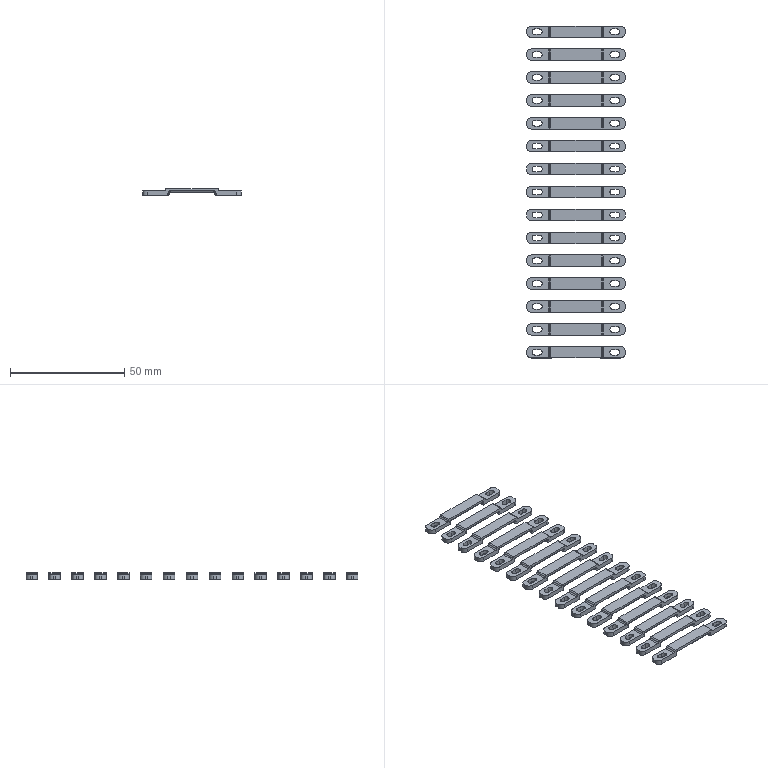NC program | NX | posted with a generic post | part box 43 x 145 x 3 mm
Lines 4404 to 5248 of 17881:
(ZLEVEL_PROFILE_COPY , TOOL : D2)
N8782 T17 M6
N8784 G54
N8786 G17 G0 G90 X-69.82 Y-18.097 S18939 M3
N8788 G43 Z30. H17
N8790 Z0.5
N8792 G94 G1 X-69.8 Y-18.064 Z0.498 F1000.
N8794 Y-15.936 Z0.386
N8796 X-69.824 Y-15.885 Z0.383
N8798 X-69.874 Y-15.845 Z0.38
N8800 X-69.901 Y-15.826 Z0.378
N8802 X-69.957 Y-15.795 Z0.375
N8804 X-70.026 Y-15.792 Z0.371
N8806 X-70.143 Y-15.846 Z0.365
N8808 X-70.2 Y-15.936 Z0.359
N8810 Y-16.021 Z0.355
N8812 Y-18.006 Z0.251
N8814 X-70.198 Y-18.07 Z0.247
N8816 X-70.147 Y-18.15 Z0.242
N8818 X-70.065 Y-18.2 Z0.237
N8820 X-69.937 Z0.231
N8822 X-69.852 Y-18.149 Z0.225
N8824 X-69.8 Y-18.064 Z0.22
N8826 Y-15.936 Z0.109
N8828 X-69.824 Y-15.885 Z0.106
N8830 X-69.874 Y-15.845 Z0.102
N8832 X-69.901 Y-15.826 Z0.101
N8834 X-69.957 Y-15.795 Z0.097
N8836 X-70.026 Y-15.792 Z0.094
N8838 X-70.143 Y-15.846 Z0.087
N8840 X-70.2 Y-15.936 Z0.081
N8842 Y-16.021 Z0.077
N8844 Y-18.006 Z-0.027
N8846 X-70.198 Y-18.07 Z-0.031
N8848 X-70.147 Y-18.15 Z-0.036
N8850 X-70.065 Y-18.2 Z-0.041
N8852 X-69.937 Z-0.047
N8854 X-69.852 Y-18.149 Z-0.053
N8856 X-69.8 Y-18.064 Z-0.058
N8858 Y-15.936 Z-0.169
N8860 X-69.824 Y-15.885 Z-0.172
N8862 X-69.874 Y-15.845 Z-0.176
N8864 X-69.901 Y-15.826 Z-0.177
N8866 X-69.957 Y-15.795 Z-0.181
N8868 X-70.026 Y-15.792 Z-0.184
N8870 X-70.143 Y-15.846 Z-0.191
N8872 X-70.2 Y-15.936 Z-0.197
N8874 Y-16. Z-0.2
N8876 Y-18.006 F1200.
N8878 G3 X-70.001 Y-18.2 R0.2
N8880 X-69.8 Y-17.985 R0.201
N8882 G1 Y-16.
N8884 X-69.799 Y-15.939
N8886 X-69.826 Y-15.883
N8888 X-69.874 Y-15.845
N8890 X-69.901 Y-15.826
N8892 G3 X-70.2 Y-16. R0.2
N8894 G1 Y-17.873 Z-0.295
N8896 X-70.199 Y-17.971 Z-0.3
N8898 X-70.183 Y-18.064 Z-0.305
N8900 X-70.164 Y-18.102 Z-0.307
N8902 X-70.155 Y-18.118 Z-0.308
N8904 X-70.129 Y-18.145 Z-0.31
N8906 X-70.058 Y-18.184 Z-0.314
N8908 X-70.022 Y-18.193 Z-0.316
N8910 X-69.999 Y-18.195 Z-0.317
N8912 X-69.951 Y-18.188 Z-0.32
N8914 X-69.886 Y-18.157 Z-0.324
N8916 X-69.861 Y-18.134 Z-0.325
N8918 X-69.843 Y-18.113 Z-0.327
N8920 X-69.816 Y-18.063 Z-0.33
N8922 X-69.808 Y-18.03 Z-0.332
N8924 X-69.8 Y-17.869 Z-0.34
N8926 Y-16.686 Z-0.4
N8928 Y-16.
N8930 X-69.799 Y-15.939
N8932 X-69.826 Y-15.883
N8934 X-69.874 Y-15.845
N8936 X-69.901 Y-15.826
N8938 G3 X-70.2 Y-16. R0.2
N8940 G1 Y-17.873 Z-0.495
N8942 X-70.199 Y-17.971 Z-0.5
N8944 X-70.183 Y-18.064 Z-0.505
N8946 X-70.164 Y-18.102 Z-0.507
N8948 X-70.155 Y-18.118 Z-0.508
N8950 X-70.129 Y-18.145 Z-0.51
N8952 X-70.058 Y-18.184 Z-0.514
N8954 X-70.022 Y-18.193 Z-0.516
N8956 X-69.999 Y-18.195 Z-0.517
N8958 X-69.951 Y-18.188 Z-0.52
N8960 X-69.886 Y-18.157 Z-0.524
N8962 X-69.861 Y-18.134 Z-0.525
N8964 X-69.843 Y-18.113 Z-0.527
N8966 X-69.816 Y-18.063 Z-0.53
N8968 X-69.808 Y-18.03 Z-0.532
N8970 X-69.8 Y-17.869 Z-0.54
N8972 Y-16.686 Z-0.6
N8974 Y-16.
N8976 X-69.799 Y-15.939
N8978 X-69.826 Y-15.883
N8980 X-69.874 Y-15.845
N8982 X-69.901 Y-15.826
N8984 G3 X-70.2 Y-16. R0.2
N8986 G1 Y-17.873 Z-0.695
N8988 X-70.199 Y-17.971 Z-0.7
N8990 X-70.183 Y-18.064 Z-0.705
N8992 X-70.164 Y-18.102 Z-0.707
N8994 X-70.155 Y-18.118 Z-0.708
N8996 X-70.129 Y-18.145 Z-0.71
N8998 X-70.058 Y-18.184 Z-0.714
N9000 X-70.022 Y-18.193 Z-0.716
N9002 X-69.999 Y-18.195 Z-0.717
N9004 X-69.951 Y-18.188 Z-0.72
N9006 X-69.886 Y-18.157 Z-0.724
N9008 X-69.861 Y-18.134 Z-0.725
N9010 X-69.843 Y-18.113 Z-0.727
N9012 X-69.816 Y-18.063 Z-0.73
N9014 X-69.808 Y-18.03 Z-0.732
N9016 X-69.8 Y-17.869 Z-0.74
N9018 Y-16.686 Z-0.8
N9020 Y-16.
N9022 X-69.799 Y-15.939
N9024 X-69.826 Y-15.883
N9026 X-69.874 Y-15.845
N9028 X-69.901 Y-15.826
N9030 G3 X-70.2 Y-16. R0.2
N9032 G1 Y-17.873 Z-0.895
N9034 X-70.199 Y-17.971 Z-0.9
N9036 X-70.183 Y-18.064 Z-0.905
N9038 X-70.164 Y-18.102 Z-0.907
N9040 X-70.155 Y-18.118 Z-0.908
N9042 X-70.129 Y-18.145 Z-0.91
N9044 X-70.058 Y-18.184 Z-0.914
N9046 X-70.022 Y-18.193 Z-0.916
N9048 X-69.999 Y-18.195 Z-0.917
N9050 X-69.951 Y-18.188 Z-0.92
N9052 X-69.886 Y-18.157 Z-0.924
N9054 X-69.861 Y-18.134 Z-0.925
N9056 X-69.843 Y-18.113 Z-0.927
N9058 X-69.816 Y-18.063 Z-0.93
N9060 X-69.808 Y-18.03 Z-0.932
N9062 X-69.8 Y-17.869 Z-0.94
N9064 Y-16.686 Z-1.
N9066 Y-16.
N9068 G3 X-70. Y-15.8 R0.2
N9070 X-70.2 Y-16. R0.2
N9072 G1 Y-16.099 Z-1.005
N9074 Y-17.873 Z-1.095
N9076 X-70.199 Y-17.971 Z-1.1
N9078 X-70.183 Y-18.064 Z-1.105
N9080 X-70.164 Y-18.102 Z-1.107
N9082 X-70.155 Y-18.118 Z-1.108
N9084 X-70.129 Y-18.145 Z-1.11
N9086 X-70.058 Y-18.184 Z-1.114
N9088 X-70.022 Y-18.193 Z-1.116
N9090 X-69.999 Y-18.195 Z-1.117
N9092 X-69.951 Y-18.188 Z-1.12
N9094 X-69.886 Y-18.157 Z-1.124
N9096 X-69.861 Y-18.134 Z-1.125
N9098 X-69.843 Y-18.113 Z-1.127
N9100 X-69.816 Y-18.063 Z-1.13
N9102 X-69.808 Y-18.03 Z-1.132
N9104 X-69.8 Y-17.869 Z-1.14
N9106 Y-16.686 Z-1.2
N9108 Y-16.
N9110 G3 X-70. Y-15.8 R0.2
N9112 X-70.2 Y-16. R0.2
N9114 G1 Y-16.099 Z-1.205
N9116 Y-17.873 Z-1.295
N9118 X-70.199 Y-17.971 Z-1.3
N9120 X-70.183 Y-18.064 Z-1.305
N9122 X-70.164 Y-18.102 Z-1.307
N9124 X-70.155 Y-18.118 Z-1.308
N9126 X-70.129 Y-18.145 Z-1.31
N9128 X-70.058 Y-18.184 Z-1.314
N9130 X-70.022 Y-18.193 Z-1.316
N9132 X-69.999 Y-18.195 Z-1.317
N9134 X-69.951 Y-18.188 Z-1.32
N9136 X-69.886 Y-18.157 Z-1.324
N9138 X-69.861 Y-18.134 Z-1.325
N9140 X-69.843 Y-18.113 Z-1.327
N9142 X-69.816 Y-18.063 Z-1.33
N9144 X-69.808 Y-18.03 Z-1.332
N9146 X-69.8 Y-17.869 Z-1.34
N9148 Y-16.686 Z-1.4
N9150 Y-16.
N9152 G3 X-70. Y-15.8 R0.2
N9154 X-70.2 Y-16. R0.2
N9156 G1 Y-16.099 Z-1.405
N9158 Y-17.873 Z-1.495
N9160 X-70.199 Y-17.971 Z-1.5
N9162 X-70.183 Y-18.064 Z-1.505
N9164 X-70.164 Y-18.102 Z-1.507
N9166 X-70.155 Y-18.118 Z-1.508
N9168 X-70.129 Y-18.145 Z-1.51
N9170 X-70.058 Y-18.184 Z-1.514
N9172 X-70.022 Y-18.193 Z-1.516
N9174 X-69.999 Y-18.195 Z-1.517
N9176 X-69.951 Y-18.188 Z-1.52
N9178 X-69.886 Y-18.157 Z-1.524
N9180 X-69.861 Y-18.134 Z-1.525
N9182 X-69.843 Y-18.113 Z-1.527
N9184 X-69.816 Y-18.063 Z-1.53
N9186 X-69.808 Y-18.03 Z-1.532
N9188 X-69.8 Y-17.869 Z-1.54
N9190 Y-16.686 Z-1.6
N9192 Y-16.
N9194 G3 X-70. Y-15.8 R0.2
N9196 X-70.2 Y-16. R0.2
N9198 G1 Y-16.099 Z-1.605
N9200 Y-17.873 Z-1.695
N9202 X-70.199 Y-17.971 Z-1.7
N9204 X-70.183 Y-18.064 Z-1.705
N9206 X-70.164 Y-18.102 Z-1.707
N9208 X-70.155 Y-18.118 Z-1.708
N9210 X-70.129 Y-18.145 Z-1.71
N9212 X-70.058 Y-18.184 Z-1.714
N9214 X-70.022 Y-18.193 Z-1.716
N9216 X-69.999 Y-18.195 Z-1.717
N9218 X-69.951 Y-18.188 Z-1.72
N9220 X-69.886 Y-18.157 Z-1.724
N9222 X-69.861 Y-18.134 Z-1.725
N9224 X-69.843 Y-18.113 Z-1.727
N9226 X-69.816 Y-18.063 Z-1.73
N9228 X-69.808 Y-18.03 Z-1.732
N9230 X-69.8 Y-17.869 Z-1.74
N9232 Y-16.686 Z-1.8
N9234 Y-16.
N9236 G3 X-70. Y-15.8 R0.2
N9238 X-70.2 Y-16. R0.2
N9240 G1 Y-16.099 Z-1.805
N9242 Y-17.873 Z-1.895
N9244 X-70.199 Y-17.971 Z-1.9
N9246 X-70.183 Y-18.064 Z-1.905
N9248 X-70.164 Y-18.102 Z-1.907
N9250 X-70.154 Y-18.118 Z-1.908
N9252 X-70.129 Y-18.145 Z-1.91
N9254 X-70.058 Y-18.184 Z-1.914
N9256 X-70.022 Y-18.193 Z-1.916
N9258 X-69.999 Y-18.195 Z-1.917
N9260 X-69.951 Y-18.188 Z-1.92
N9262 X-69.886 Y-18.157 Z-1.924
N9264 X-69.861 Y-18.134 Z-1.925
N9266 X-69.843 Y-18.113 Z-1.927
N9268 X-69.816 Y-18.063 Z-1.93
N9270 X-69.808 Y-18.03 Z-1.932
N9272 X-69.8 Y-17.869 Z-1.94
N9274 Y-16.686 Z-2.
N9276 Y-16.
N9278 G3 X-70. Y-15.8 R0.2
N9280 X-70.2 Y-16.002 R0.2
N9282 G1 Y-18.006
N9284 G3 X-70.001 Y-18.2 R0.2
N9286 X-69.8 Y-17.985 R0.201
N9288 G1 Y-16.686
N9290 Z-1.5
N9292 G0 Z30.
N9294 X-59.82 Y-18.097
N9296 Z0.5
N9298 G1 X-59.8 Y-18.064 Z0.498 F1000.
N9300 Y-15.936 Z0.386
N9302 X-59.824 Y-15.885 Z0.383
N9304 X-59.874 Y-15.845 Z0.38
N9306 X-59.901 Y-15.826 Z0.378
N9308 X-59.957 Y-15.795 Z0.375
N9310 X-60.026 Y-15.792 Z0.371
N9312 X-60.143 Y-15.846 Z0.365
N9314 X-60.2 Y-15.936 Z0.359
N9316 Y-16.021 Z0.355
N9318 Y-18.006 Z0.251
N9320 X-60.198 Y-18.07 Z0.247
N9322 X-60.147 Y-18.15 Z0.242
N9324 X-60.065 Y-18.2 Z0.237
N9326 X-59.937 Z0.231
N9328 X-59.852 Y-18.149 Z0.225
N9330 X-59.8 Y-18.064 Z0.22
N9332 Y-15.936 Z0.109
N9334 X-59.824 Y-15.885 Z0.106
N9336 X-59.874 Y-15.845 Z0.102
N9338 X-59.901 Y-15.826 Z0.101
N9340 X-59.957 Y-15.795 Z0.097
N9342 X-60.026 Y-15.792 Z0.094
N9344 X-60.143 Y-15.846 Z0.087
N9346 X-60.2 Y-15.936 Z0.081
N9348 Y-16.021 Z0.077
N9350 Y-18.006 Z-0.027
N9352 X-60.198 Y-18.07 Z-0.031
N9354 X-60.147 Y-18.15 Z-0.036
N9356 X-60.065 Y-18.2 Z-0.041
N9358 X-59.937 Z-0.047
N9360 X-59.852 Y-18.149 Z-0.053
N9362 X-59.8 Y-18.064 Z-0.058
N9364 Y-15.936 Z-0.169
N9366 X-59.824 Y-15.885 Z-0.172
N9368 X-59.874 Y-15.845 Z-0.176
N9370 X-59.901 Y-15.826 Z-0.177
N9372 X-59.957 Y-15.795 Z-0.181
N9374 X-60.026 Y-15.792 Z-0.184
N9376 X-60.143 Y-15.846 Z-0.191
N9378 X-60.2 Y-15.936 Z-0.197
N9380 Y-16. Z-0.2
N9382 Y-18.006 F1200.
N9384 G3 X-60.001 Y-18.2 R0.2
N9386 X-59.8 Y-17.985 R0.201
N9388 G1 Y-16.
N9390 X-59.799 Y-15.939
N9392 X-59.826 Y-15.883
N9394 X-59.874 Y-15.845
N9396 X-59.901 Y-15.826
N9398 G3 X-60.2 Y-16. R0.2
N9400 G1 Y-17.873 Z-0.295
N9402 X-60.199 Y-17.971 Z-0.3
N9404 X-60.183 Y-18.064 Z-0.305
N9406 X-60.164 Y-18.102 Z-0.307
N9408 X-60.155 Y-18.118 Z-0.308
N9410 X-60.129 Y-18.145 Z-0.31
N9412 X-60.058 Y-18.184 Z-0.314
N9414 X-60.022 Y-18.193 Z-0.316
N9416 X-59.999 Y-18.195 Z-0.317
N9418 X-59.951 Y-18.188 Z-0.32
N9420 X-59.886 Y-18.157 Z-0.324
N9422 X-59.861 Y-18.134 Z-0.325
N9424 X-59.843 Y-18.113 Z-0.327
N9426 X-59.816 Y-18.063 Z-0.33
N9428 X-59.808 Y-18.03 Z-0.332
N9430 X-59.8 Y-17.869 Z-0.34
N9432 Y-16.686 Z-0.4
N9434 Y-16.
N9436 X-59.799 Y-15.939
N9438 X-59.826 Y-15.883
N9440 X-59.874 Y-15.845
N9442 X-59.901 Y-15.826
N9444 G3 X-60.2 Y-16. R0.2
N9446 G1 Y-17.873 Z-0.495
N9448 X-60.199 Y-17.971 Z-0.5
N9450 X-60.183 Y-18.064 Z-0.505
N9452 X-60.164 Y-18.102 Z-0.507
N9454 X-60.155 Y-18.118 Z-0.508
N9456 X-60.129 Y-18.145 Z-0.51
N9458 X-60.058 Y-18.184 Z-0.514
N9460 X-60.022 Y-18.193 Z-0.516
N9462 X-59.999 Y-18.195 Z-0.517
N9464 X-59.951 Y-18.188 Z-0.52
N9466 X-59.886 Y-18.157 Z-0.524
N9468 X-59.861 Y-18.134 Z-0.525
N9470 X-59.843 Y-18.113 Z-0.527
N9472 X-59.816 Y-18.063 Z-0.53
N9474 X-59.808 Y-18.03 Z-0.532
N9476 X-59.8 Y-17.869 Z-0.54
N9478 Y-16.686 Z-0.6
N9480 Y-16.
N9482 X-59.799 Y-15.939
N9484 X-59.826 Y-15.883
N9486 X-59.874 Y-15.845
N9488 X-59.901 Y-15.826
N9490 G3 X-60.2 Y-16. R0.2
N9492 G1 Y-17.873 Z-0.695
N9494 X-60.199 Y-17.971 Z-0.7
N9496 X-60.183 Y-18.064 Z-0.705
N9498 X-60.164 Y-18.102 Z-0.707
N9500 X-60.155 Y-18.118 Z-0.708
N9502 X-60.129 Y-18.145 Z-0.71
N9504 X-60.058 Y-18.184 Z-0.714
N9506 X-60.022 Y-18.193 Z-0.716
N9508 X-59.999 Y-18.195 Z-0.717
N9510 X-59.951 Y-18.188 Z-0.72
N9512 X-59.886 Y-18.157 Z-0.724
N9514 X-59.861 Y-18.134 Z-0.725
N9516 X-59.843 Y-18.113 Z-0.727
N9518 X-59.816 Y-18.063 Z-0.73
N9520 X-59.808 Y-18.03 Z-0.732
N9522 X-59.8 Y-17.869 Z-0.74
N9524 Y-16.686 Z-0.8
N9526 Y-16.
N9528 X-59.799 Y-15.939
N9530 X-59.826 Y-15.883
N9532 X-59.874 Y-15.845
N9534 X-59.901 Y-15.826
N9536 G3 X-60.2 Y-16. R0.2
N9538 G1 Y-17.873 Z-0.895
N9540 X-60.199 Y-17.971 Z-0.9
N9542 X-60.183 Y-18.064 Z-0.905
N9544 X-60.164 Y-18.102 Z-0.907
N9546 X-60.155 Y-18.118 Z-0.908
N9548 X-60.129 Y-18.145 Z-0.91
N9550 X-60.058 Y-18.184 Z-0.914
N9552 X-60.022 Y-18.193 Z-0.916
N9554 X-59.999 Y-18.195 Z-0.917
N9556 X-59.951 Y-18.188 Z-0.92
N9558 X-59.886 Y-18.157 Z-0.924
N9560 X-59.861 Y-18.134 Z-0.925
N9562 X-59.843 Y-18.113 Z-0.927
N9564 X-59.816 Y-18.063 Z-0.93
N9566 X-59.808 Y-18.03 Z-0.932
N9568 X-59.8 Y-17.869 Z-0.94
N9570 Y-16.784 Z-0.995
N9572 Y-16.686 Z-1.
N9574 Y-16.
N9576 G3 X-60. Y-15.8 R0.2
N9578 X-60.2 Y-16. R0.2
N9580 G1 Y-16.296 Z-1.015
N9582 Y-17.873 Z-1.095
N9584 X-60.199 Y-17.971 Z-1.1
N9586 X-60.183 Y-18.064 Z-1.105
N9588 X-60.164 Y-18.102 Z-1.107
N9590 X-60.155 Y-18.118 Z-1.108
N9592 X-60.129 Y-18.145 Z-1.11
N9594 X-60.058 Y-18.184 Z-1.114
N9596 X-60.022 Y-18.193 Z-1.116
N9598 X-59.999 Y-18.195 Z-1.117
N9600 X-59.951 Y-18.188 Z-1.12
N9602 X-59.886 Y-18.157 Z-1.124
N9604 X-59.861 Y-18.134 Z-1.125
N9606 X-59.843 Y-18.113 Z-1.127
N9608 X-59.816 Y-18.063 Z-1.13
N9610 X-59.808 Y-18.03 Z-1.132
N9612 X-59.8 Y-17.869 Z-1.14
N9614 Y-16.784 Z-1.195
N9616 Y-16.686 Z-1.2
N9618 Y-16.
N9620 G3 X-60. Y-15.8 R0.2
N9622 X-60.2 Y-16. R0.2
N9624 G1 Y-16.296 Z-1.215
N9626 Y-17.873 Z-1.295
N9628 X-60.199 Y-17.971 Z-1.3
N9630 X-60.183 Y-18.064 Z-1.305
N9632 X-60.164 Y-18.102 Z-1.307
N9634 X-60.155 Y-18.118 Z-1.308
N9636 X-60.129 Y-18.145 Z-1.31
N9638 X-60.058 Y-18.184 Z-1.314
N9640 X-60.022 Y-18.193 Z-1.316
N9642 X-59.999 Y-18.195 Z-1.317
N9644 X-59.951 Y-18.188 Z-1.32
N9646 X-59.886 Y-18.157 Z-1.324
N9648 X-59.861 Y-18.134 Z-1.325
N9650 X-59.843 Y-18.113 Z-1.327
N9652 X-59.816 Y-18.063 Z-1.33
N9654 X-59.808 Y-18.03 Z-1.332
N9656 X-59.8 Y-17.869 Z-1.34
N9658 Y-16.784 Z-1.395
N9660 Y-16.686 Z-1.4
N9662 Y-16.
N9664 G3 X-60. Y-15.8 R0.2
N9666 X-60.2 Y-16. R0.2
N9668 G1 Y-16.296 Z-1.415
N9670 Y-17.873 Z-1.495
N9672 X-60.199 Y-17.971 Z-1.5
N9674 X-60.183 Y-18.064 Z-1.505
N9676 X-60.164 Y-18.102 Z-1.507
N9678 X-60.155 Y-18.118 Z-1.508
N9680 X-60.129 Y-18.145 Z-1.51
N9682 X-60.058 Y-18.184 Z-1.514
N9684 X-60.022 Y-18.193 Z-1.516
N9686 X-59.999 Y-18.195 Z-1.517
N9688 X-59.951 Y-18.188 Z-1.52
N9690 X-59.886 Y-18.157 Z-1.524
N9692 X-59.861 Y-18.134 Z-1.525
N9694 X-59.843 Y-18.113 Z-1.527
N9696 X-59.816 Y-18.063 Z-1.53
N9698 X-59.808 Y-18.03 Z-1.532
N9700 X-59.8 Y-17.869 Z-1.54
N9702 Y-16.784 Z-1.595
N9704 Y-16.686 Z-1.6
N9706 Y-16.
N9708 G3 X-60. Y-15.8 R0.2
N9710 X-60.2 Y-16. R0.2
N9712 G1 Y-16.296 Z-1.615
N9714 Y-17.873 Z-1.695
N9716 X-60.199 Y-17.971 Z-1.7
N9718 X-60.183 Y-18.064 Z-1.705
N9720 X-60.164 Y-18.102 Z-1.707
N9722 X-60.155 Y-18.118 Z-1.708
N9724 X-60.129 Y-18.145 Z-1.71
N9726 X-60.058 Y-18.184 Z-1.714
N9728 X-60.022 Y-18.193 Z-1.716
N9730 X-59.999 Y-18.195 Z-1.717
N9732 X-59.951 Y-18.188 Z-1.72
N9734 X-59.886 Y-18.157 Z-1.724
N9736 X-59.861 Y-18.134 Z-1.725
N9738 X-59.843 Y-18.113 Z-1.727
N9740 X-59.816 Y-18.063 Z-1.73
N9742 X-59.808 Y-18.03 Z-1.732
N9744 X-59.8 Y-17.869 Z-1.74
N9746 Y-16.784 Z-1.795
N9748 Y-16.686 Z-1.8
N9750 Y-16.
N9752 G3 X-60. Y-15.8 R0.2
N9754 X-60.2 Y-16. R0.2
N9756 G1 Y-16.296 Z-1.815
N9758 Y-17.873 Z-1.895
N9760 X-60.199 Y-17.971 Z-1.9
N9762 X-60.183 Y-18.064 Z-1.905
N9764 X-60.164 Y-18.102 Z-1.907
N9766 X-60.154 Y-18.118 Z-1.908
N9768 X-60.129 Y-18.145 Z-1.91
N9770 X-60.058 Y-18.184 Z-1.914
N9772 X-60.022 Y-18.193 Z-1.916
N9774 X-59.999 Y-18.195 Z-1.917
N9776 X-59.951 Y-18.188 Z-1.92
N9778 X-59.886 Y-18.157 Z-1.924
N9780 X-59.861 Y-18.134 Z-1.925
N9782 X-59.843 Y-18.113 Z-1.927
N9784 X-59.816 Y-18.063 Z-1.93
N9786 X-59.808 Y-18.03 Z-1.932
N9788 X-59.8 Y-17.869 Z-1.94
N9790 Y-16.784 Z-1.995
N9792 Y-16.686 Z-2.
N9794 Y-16.
N9796 G3 X-60. Y-15.8 R0.2
N9798 X-60.2 Y-16.002 R0.2
N9800 G1 Y-18.006
N9802 G3 X-60.001 Y-18.2 R0.2
N9804 X-59.8 Y-17.985 R0.201
N9806 G1 Y-16.686
N9808 Z-1.5
N9810 G0 Z30.
N9812 X-49.82 Y-18.097
N9814 Z0.5
N9816 G1 X-49.8 Y-18.064 Z0.498 F1000.
N9818 Y-15.936 Z0.386
N9820 X-49.824 Y-15.885 Z0.383
N9822 X-49.874 Y-15.845 Z0.38
N9824 X-49.901 Y-15.826 Z0.378
N9826 X-49.957 Y-15.795 Z0.375
N9828 X-50.026 Y-15.792 Z0.371
N9830 X-50.143 Y-15.846 Z0.365
N9832 X-50.2 Y-15.936 Z0.359
N9834 Y-16.021 Z0.355
N9836 Y-18.006 Z0.251
N9838 X-50.198 Y-18.07 Z0.247
N9840 X-50.147 Y-18.15 Z0.242
N9842 X-50.065 Y-18.2 Z0.237
N9844 X-49.937 Z0.231
N9846 X-49.852 Y-18.149 Z0.225
N9848 X-49.8 Y-18.064 Z0.22
N9850 Y-15.936 Z0.109
N9852 X-49.824 Y-15.885 Z0.106
N9854 X-49.874 Y-15.845 Z0.102
N9856 X-49.901 Y-15.826 Z0.101
N9858 X-49.957 Y-15.795 Z0.097
N9860 X-50.026 Y-15.792 Z0.094
N9862 X-50.143 Y-15.846 Z0.087
N9864 X-50.2 Y-15.936 Z0.081
N9866 Y-16.021 Z0.077
N9868 Y-18.006 Z-0.027
N9870 X-50.198 Y-18.07 Z-0.031
N9872 X-50.147 Y-18.15 Z-0.036
N9874 X-50.065 Y-18.2 Z-0.041
N9876 X-49.937 Z-0.047
N9878 X-49.852 Y-18.149 Z-0.053
N9880 X-49.8 Y-18.064 Z-0.058
N9882 Y-15.936 Z-0.169
N9884 X-49.824 Y-15.885 Z-0.172
N9886 X-49.874 Y-15.845 Z-0.176
N9888 X-49.901 Y-15.826 Z-0.177
N9890 X-49.957 Y-15.795 Z-0.181
N9892 X-50.026 Y-15.792 Z-0.184
N9894 X-50.143 Y-15.846 Z-0.191
N9896 X-50.2 Y-15.936 Z-0.197
N9898 Y-16. Z-0.2
N9900 Y-18.006 F1200.
N9902 G3 X-50.001 Y-18.2 R0.2
N9904 X-49.8 Y-17.985 R0.201
N9906 G1 Y-16.
N9908 X-49.799 Y-15.939
N9910 X-49.826 Y-15.883
N9912 X-49.874 Y-15.845
N9914 X-49.901 Y-15.826
N9916 G3 X-50.2 Y-16. R0.2
N9918 G1 Y-17.873 Z-0.295
N9920 X-50.199 Y-17.971 Z-0.3
N9922 X-50.183 Y-18.064 Z-0.305
N9924 X-50.164 Y-18.102 Z-0.307
N9926 X-50.155 Y-18.118 Z-0.308
N9928 X-50.129 Y-18.145 Z-0.31
N9930 X-50.058 Y-18.184 Z-0.314
N9932 X-50.022 Y-18.193 Z-0.316
N9934 X-49.999 Y-18.195 Z-0.317
N9936 X-49.951 Y-18.188 Z-0.32
N9938 X-49.886 Y-18.157 Z-0.324
N9940 X-49.861 Y-18.134 Z-0.325
N9942 X-49.843 Y-18.113 Z-0.327
N9944 X-49.816 Y-18.063 Z-0.33
N9946 X-49.808 Y-18.03 Z-0.332
N9948 X-49.8 Y-17.869 Z-0.34
N9950 Y-16.686 Z-0.4
N9952 Y-16.
N9954 X-49.799 Y-15.939
N9956 X-49.826 Y-15.883
N9958 X-49.874 Y-15.845
N9960 X-49.901 Y-15.826
N9962 G3 X-50.2 Y-16. R0.2
N9964 G1 Y-17.873 Z-0.495
N9966 X-50.199 Y-17.971 Z-0.5
N9968 X-50.183 Y-18.064 Z-0.505
N9970 X-50.164 Y-18.102 Z-0.507
N9972 X-50.155 Y-18.118 Z-0.508
N9974 X-50.129 Y-18.145 Z-0.51
N9976 X-50.058 Y-18.184 Z-0.514
N9978 X-50.022 Y-18.193 Z-0.516
N9980 X-49.999 Y-18.195 Z-0.517
N9982 X-49.951 Y-18.188 Z-0.52
N9984 X-49.886 Y-18.157 Z-0.524
N9986 X-49.861 Y-18.134 Z-0.525
N9988 X-49.843 Y-18.113 Z-0.527
N9990 X-49.816 Y-18.063 Z-0.53
N9992 X-49.808 Y-18.03 Z-0.532
N9994 X-49.8 Y-17.869 Z-0.54
N9996 Y-16.686 Z-0.6
N9998 Y-16.
N10000 X-49.799 Y-15.939
N10002 X-49.826 Y-15.883
N10004 X-49.874 Y-15.845
N10006 X-49.901 Y-15.826
N10008 G3 X-50.2 Y-16. R0.2
N10010 G1 Y-17.873 Z-0.695
N10012 X-50.199 Y-17.971 Z-0.7
N10014 X-50.183 Y-18.064 Z-0.705
N10016 X-50.164 Y-18.102 Z-0.707
N10018 X-50.155 Y-18.118 Z-0.708
N10020 X-50.129 Y-18.145 Z-0.71
N10022 X-50.058 Y-18.184 Z-0.714
N10024 X-50.022 Y-18.193 Z-0.716
N10026 X-49.999 Y-18.195 Z-0.717
N10028 X-49.951 Y-18.188 Z-0.72
N10030 X-49.886 Y-18.157 Z-0.724
N10032 X-49.861 Y-18.134 Z-0.725
N10034 X-49.843 Y-18.113 Z-0.727
N10036 X-49.816 Y-18.063 Z-0.73
N10038 X-49.808 Y-18.03 Z-0.732
N10040 X-49.8 Y-17.869 Z-0.74
N10042 Y-16.686 Z-0.8
N10044 Y-16.
N10046 X-49.799 Y-15.939
N10048 X-49.826 Y-15.883
N10050 X-49.874 Y-15.845
N10052 X-49.901 Y-15.826
N10054 G3 X-50.2 Y-16. R0.2
N10056 G1 Y-17.873 Z-0.895
N10058 X-50.199 Y-17.971 Z-0.9
N10060 X-50.183 Y-18.064 Z-0.905
N10062 X-50.164 Y-18.102 Z-0.907
N10064 X-50.155 Y-18.118 Z-0.908
N10066 X-50.129 Y-18.145 Z-0.91
N10068 X-50.058 Y-18.184 Z-0.914
N10070 X-50.022 Y-18.193 Z-0.916
N10072 X-49.999 Y-18.195 Z-0.917
N10074 X-49.951 Y-18.188 Z-0.92
N10076 X-49.886 Y-18.157 Z-0.924
N10078 X-49.861 Y-18.134 Z-0.925
N10080 X-49.843 Y-18.113 Z-0.927
N10082 X-49.816 Y-18.063 Z-0.93
N10084 X-49.808 Y-18.03 Z-0.932
N10086 X-49.8 Y-17.869 Z-0.94
N10088 Y-16.784 Z-0.995
N10090 Y-16.686 Z-1.
N10092 Y-16.
N10094 G3 X-50. Y-15.8 R0.2
N10096 X-50.2 Y-16. R0.2
N10098 G1 Y-16.099 Z-1.005
N10100 Y-17.873 Z-1.095
N10102 X-50.199 Y-17.971 Z-1.1
N10104 X-50.183 Y-18.064 Z-1.105
N10106 X-50.164 Y-18.102 Z-1.107
N10108 X-50.155 Y-18.118 Z-1.108
N10110 X-50.129 Y-18.145 Z-1.11
N10112 X-50.058 Y-18.184 Z-1.114
N10114 X-50.022 Y-18.193 Z-1.116
N10116 X-49.999 Y-18.195 Z-1.117
N10118 X-49.951 Y-18.188 Z-1.12
N10120 X-49.886 Y-18.157 Z-1.124
N10122 X-49.861 Y-18.134 Z-1.125
N10124 X-49.843 Y-18.113 Z-1.127
N10126 X-49.816 Y-18.063 Z-1.13
N10128 X-49.808 Y-18.03 Z-1.132
N10130 X-49.8 Y-17.869 Z-1.14
N10132 Y-16.784 Z-1.195
N10134 Y-16.686 Z-1.2
N10136 Y-16.
N10138 G3 X-50. Y-15.8 R0.2
N10140 X-50.2 Y-16. R0.2
N10142 G1 Y-16.099 Z-1.205
N10144 Y-17.873 Z-1.295
N10146 X-50.199 Y-17.971 Z-1.3
N10148 X-50.183 Y-18.064 Z-1.305
N10150 X-50.164 Y-18.102 Z-1.307
N10152 X-50.155 Y-18.118 Z-1.308
N10154 X-50.129 Y-18.145 Z-1.31
N10156 X-50.058 Y-18.184 Z-1.314
N10158 X-50.022 Y-18.193 Z-1.316
N10160 X-49.999 Y-18.195 Z-1.317
N10162 X-49.951 Y-18.188 Z-1.32
N10164 X-49.886 Y-18.157 Z-1.324
N10166 X-49.861 Y-18.134 Z-1.325
N10168 X-49.843 Y-18.113 Z-1.327
N10170 X-49.816 Y-18.063 Z-1.33
N10172 X-49.808 Y-18.03 Z-1.332
N10174 X-49.8 Y-17.869 Z-1.34
N10176 Y-16.784 Z-1.395
N10178 Y-16.686 Z-1.4
N10180 Y-16.
N10182 G3 X-50. Y-15.8 R0.2
N10184 X-50.2 Y-16. R0.2
N10186 G1 Y-16.099 Z-1.405
N10188 Y-17.873 Z-1.495
N10190 X-50.199 Y-17.971 Z-1.5
N10192 X-50.183 Y-18.064 Z-1.505
N10194 X-50.164 Y-18.102 Z-1.507
N10196 X-50.155 Y-18.118 Z-1.508
N10198 X-50.129 Y-18.145 Z-1.51
N10200 X-50.058 Y-18.184 Z-1.514
N10202 X-50.022 Y-18.193 Z-1.516
N10204 X-49.999 Y-18.195 Z-1.517
N10206 X-49.951 Y-18.188 Z-1.52
N10208 X-49.886 Y-18.157 Z-1.524
N10210 X-49.861 Y-18.134 Z-1.525
N10212 X-49.843 Y-18.113 Z-1.527
N10214 X-49.816 Y-18.063 Z-1.53
N10216 X-49.808 Y-18.03 Z-1.532
N10218 X-49.8 Y-17.869 Z-1.54
N10220 Y-16.784 Z-1.595
N10222 Y-16.686 Z-1.6
N10224 Y-16.
N10226 G3 X-50. Y-15.8 R0.2
N10228 X-50.2 Y-16. R0.2
N10230 G1 Y-16.099 Z-1.605
N10232 Y-17.873 Z-1.695
N10234 X-50.199 Y-17.971 Z-1.7
N10236 X-50.183 Y-18.064 Z-1.705
N10238 X-50.164 Y-18.102 Z-1.707
N10240 X-50.155 Y-18.118 Z-1.708
N10242 X-50.129 Y-18.145 Z-1.71
N10244 X-50.058 Y-18.184 Z-1.714
N10246 X-50.022 Y-18.193 Z-1.716
N10248 X-49.999 Y-18.195 Z-1.717
N10250 X-49.951 Y-18.188 Z-1.72
N10252 X-49.886 Y-18.157 Z-1.724
N10254 X-49.861 Y-18.134 Z-1.725
N10256 X-49.843 Y-18.113 Z-1.727
N10258 X-49.816 Y-18.063 Z-1.73
N10260 X-49.808 Y-18.03 Z-1.732
N10262 X-49.8 Y-17.869 Z-1.74
N10264 Y-16.784 Z-1.795
N10266 Y-16.686 Z-1.8
N10268 Y-16.
N10270 G3 X-50. Y-15.8 R0.2
N10272 X-50.2 Y-16. R0.2
N10274 G1 Y-16.099 Z-1.805
N10276 Y-17.873 Z-1.895
N10278 X-50.199 Y-17.971 Z-1.9
N10280 X-50.183 Y-18.064 Z-1.905
N10282 X-50.164 Y-18.102 Z-1.907
N10284 X-50.154 Y-18.118 Z-1.908
N10286 X-50.129 Y-18.145 Z-1.91
N10288 X-50.058 Y-18.184 Z-1.914
N10290 X-50.022 Y-18.193 Z-1.916
N10292 X-49.999 Y-18.195 Z-1.917
N10294 X-49.951 Y-18.188 Z-1.92
N10296 X-49.886 Y-18.157 Z-1.924
N10298 X-49.861 Y-18.134 Z-1.925
N10300 X-49.843 Y-18.113 Z-1.927
N10302 X-49.816 Y-18.063 Z-1.93
N10304 X-49.808 Y-18.03 Z-1.932
N10306 X-49.8 Y-17.869 Z-1.94
N10308 Y-16.784 Z-1.995
N10310 Y-16.686 Z-2.
N10312 Y-16.
N10314 G3 X-50. Y-15.8 R0.2
N10316 X-50.2 Y-16.002 R0.2
N10318 G1 Y-18.006
N10320 G3 X-50.001 Y-18.2 R0.2
N10322 X-49.8 Y-17.985 R0.201
N10324 G1 Y-16.686
N10326 Z-1.5
N10328 G0 Z30.
N10330 X-39.82 Y-18.097
N10332 Z0.5
N10334 G1 X-39.8 Y-18.064 Z0.498 F1000.
N10336 Y-15.936 Z0.386
N10338 X-39.824 Y-15.885 Z0.383
N10340 X-39.874 Y-15.845 Z0.38
N10342 X-39.901 Y-15.826 Z0.378
N10344 X-39.957 Y-15.795 Z0.375
N10346 X-40.026 Y-15.792 Z0.371
N10348 X-40.143 Y-15.846 Z0.365
N10350 X-40.2 Y-15.936 Z0.359
N10352 Y-16.021 Z0.355
N10354 Y-18.006 Z0.251
N10356 X-40.198 Y-18.07 Z0.247
N10358 X-40.147 Y-18.15 Z0.242
N10360 X-40.065 Y-18.2 Z0.237
N10362 X-39.937 Z0.231
N10364 X-39.852 Y-18.149 Z0.225
N10366 X-39.8 Y-18.064 Z0.22
N10368 Y-15.936 Z0.109
N10370 X-39.824 Y-15.885 Z0.106
N10372 X-39.874 Y-15.845 Z0.102
N10374 X-39.901 Y-15.826 Z0.101
N10376 X-39.957 Y-15.795 Z0.097
N10378 X-40.026 Y-15.792 Z0.094
N10380 X-40.143 Y-15.846 Z0.087
N10382 X-40.2 Y-15.936 Z0.081
N10384 Y-16.021 Z0.077
N10386 Y-18.006 Z-0.027
N10388 X-40.198 Y-18.07 Z-0.031
N10390 X-40.147 Y-18.15 Z-0.036
N10392 X-40.065 Y-18.2 Z-0.041
N10394 X-39.937 Z-0.047
N10396 X-39.852 Y-18.149 Z-0.053
N10398 X-39.8 Y-18.064 Z-0.058
N10400 Y-15.936 Z-0.169
N10402 X-39.824 Y-15.885 Z-0.172
N10404 X-39.874 Y-15.845 Z-0.176
N10406 X-39.901 Y-15.826 Z-0.177
N10408 X-39.957 Y-15.795 Z-0.181
N10410 X-40.026 Y-15.792 Z-0.184
N10412 X-40.143 Y-15.846 Z-0.191
N10414 X-40.2 Y-15.936 Z-0.197
N10416 Y-16. Z-0.2
N10418 Y-18.006 F1200.
N10420 G3 X-40.001 Y-18.2 R0.2
N10422 X-39.8 Y-17.985 R0.201
N10424 G1 Y-16.
N10426 X-39.799 Y-15.939
N10428 X-39.826 Y-15.883
N10430 X-39.874 Y-15.845
N10432 X-39.901 Y-15.826
N10434 G3 X-40.2 Y-16. R0.2
N10436 G1 Y-17.873 Z-0.295
N10438 X-40.199 Y-17.971 Z-0.3
N10440 X-40.183 Y-18.064 Z-0.305
N10442 X-40.164 Y-18.102 Z-0.307
N10444 X-40.155 Y-18.118 Z-0.308
N10446 X-40.129 Y-18.145 Z-0.31
N10448 X-40.058 Y-18.184 Z-0.314
N10450 X-40.022 Y-18.193 Z-0.316
N10452 X-39.999 Y-18.195 Z-0.317
N10454 X-39.951 Y-18.188 Z-0.32
N10456 X-39.886 Y-18.157 Z-0.324
N10458 X-39.861 Y-18.134 Z-0.325
N10460 X-39.843 Y-18.113 Z-0.327
N10462 X-39.816 Y-18.063 Z-0.33
N10464 X-39.808 Y-18.03 Z-0.332